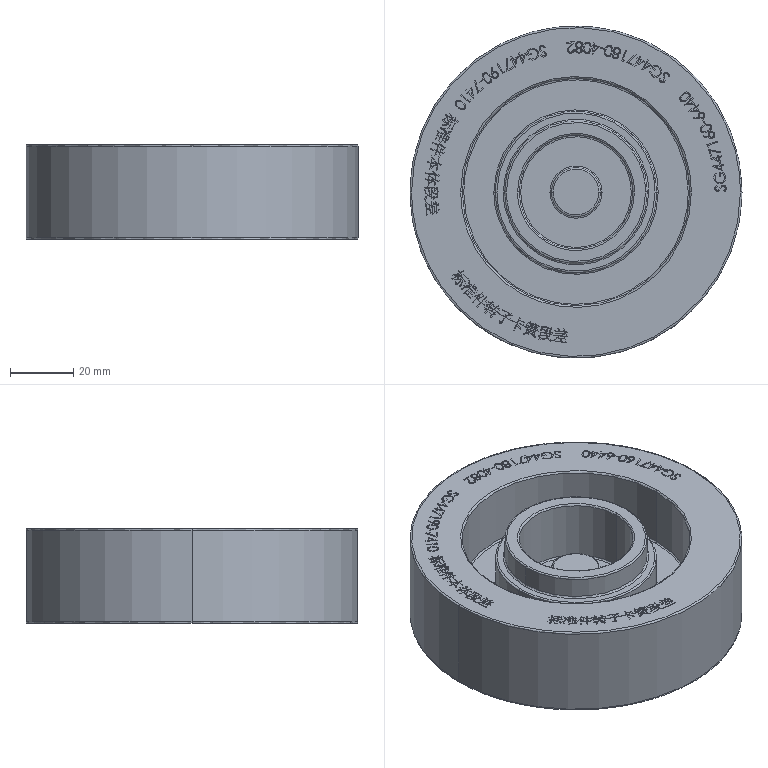Part | STEP file | Seat-PN_0001 | 1 solid | 1382 faces | box 105 x 105 x 30 mm | volume 196684 mm3 | plane 959 | spline 407 | cylinder 16 | commonest cylinder face diameters 5 x4 15.5 x2 36 x2 45 x2 51 x2 72 x2